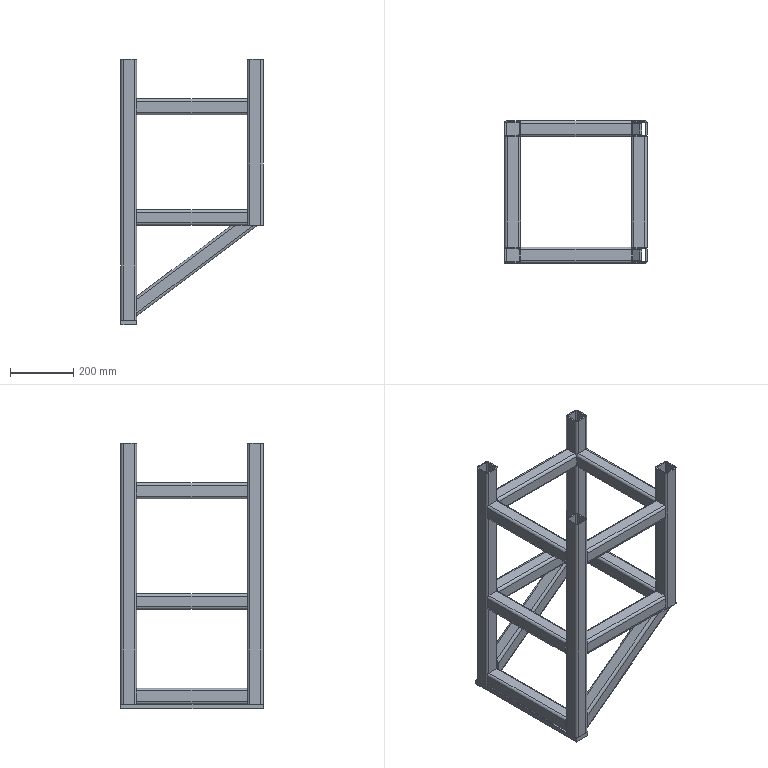Part | SolidWorks | features WeldCornerFeat 2, WeldMemberFeat 2, 3DProfileFeature 1, ICE 1, WeldmentFeature 1 | 16 solids | 276 faces | box 450 x 450 x 839 mm | volume 4973031 mm3 | plane 156 | cylinder 120 | commonest cylinder face diameters 8 x60 16 x60